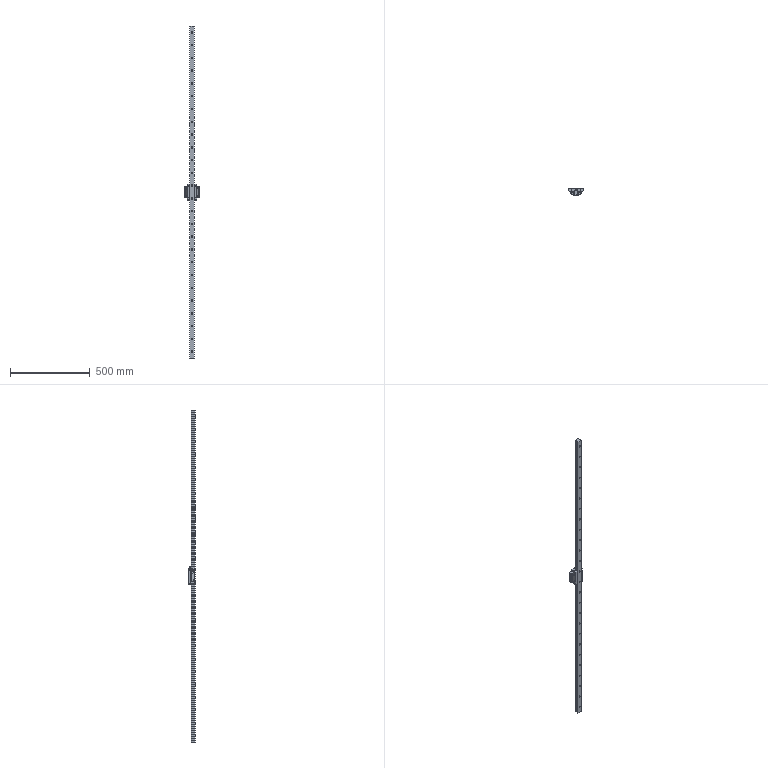Part | SolidWorks | features LocalLPattern 1 | 7 solids | 982 faces | box 90 x 42.01 x 2080 mm | volume 1460108 mm3 | plane 613 | cylinder 192 | spline 119 | torus 25 | cone 23 | sphere 10 | commonest cylinder face diameters 9 x52 14 x52 2.822 x36 4.26 x12 0.575 x8 4.788 x8